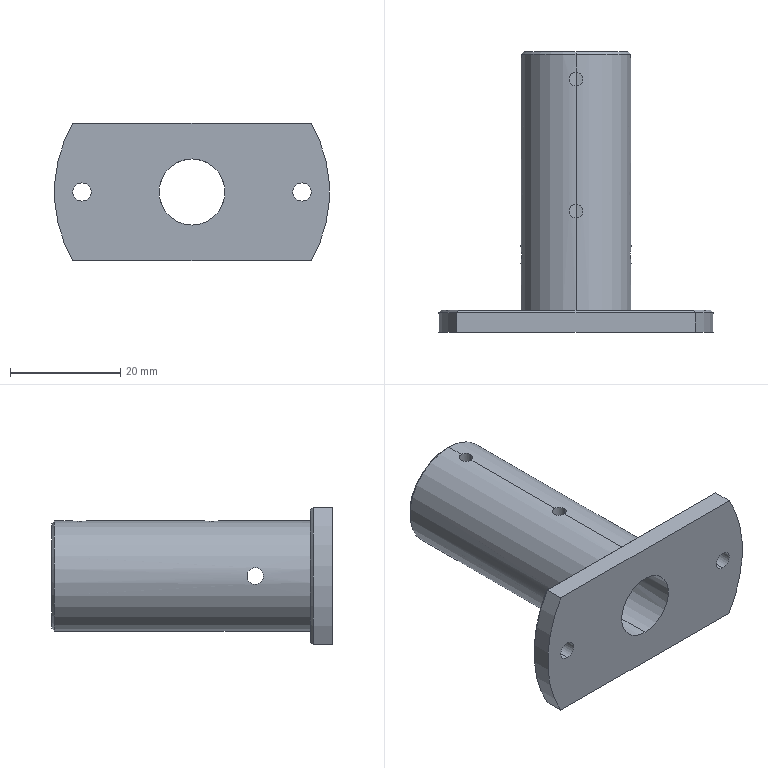Part | SolidWorks | features 3DProfileFeature 2, HoleWzd 2, ICE 2, Chamfer 1, Revolution 1 | 1 solid | 31 faces | box 50 x 51 x 25 mm | volume 13586 mm3 | cylinder 18 | plane 7 | cone 6 | commonest cylinder face diameters 2.5 x4 3 x4 3.3 x4 12 x2 20 x2 50 x2
STEP:
#1=CARTESIAN_POINT('',(-9.887,14.,1.5));
#2=VERTEX_POINT('',#1);
#3=CARTESIAN_POINT('',(-9.887,14.,-1.5));
#4=VERTEX_POINT('',#3);
#5=CARTESIAN_POINT('',(-9.887,14.,1.5));
#6=CARTESIAN_POINT('',(-9.887,13.804,1.5));
#7=CARTESIAN_POINT('',(-9.893,13.607,1.461));
#8=CARTESIAN_POINT('',(-9.914,13.245,1.311));
#9=CARTESIAN_POINT('',(-9.929,13.078,1.2));
#10=CARTESIAN_POINT('',(-9.951,12.871,0.9923));
#11=CARTESIAN_POINT('',(-9.958,12.808,0.9152));
#12=CARTESIAN_POINT('',(-9.972,12.699,0.7525));
#13=CARTESIAN_POINT('',(-9.978,12.653,0.6665));
#14=CARTESIAN_POINT('',(-9.994,12.539,0.394));
#15=CARTESIAN_POINT('',(-10.,12.5,0.1992));
#16=CARTESIAN_POINT('',(-10.,12.5,-0.09815));
#17=CARTESIAN_POINT('',(-9.999,12.51,-0.1957));
#18=CARTESIAN_POINT('',(-9.993,12.548,-0.3876));
#19=CARTESIAN_POINT('',(-9.989,12.577,-0.4831));
#20=CARTESIAN_POINT('',(-9.978,12.652,-0.6646));
#21=CARTESIAN_POINT('',(-9.972,12.698,-0.7507));
#22=CARTESIAN_POINT('',(-9.958,12.806,-0.9138));
#23=CARTESIAN_POINT('',(-9.951,12.87,-0.9909));
#24=CARTESIAN_POINT('',(-9.929,13.077,-1.198));
#25=CARTESIAN_POINT('',(-9.914,13.244,-1.31));
#26=CARTESIAN_POINT('',(-9.893,13.604,-1.46));
#27=CARTESIAN_POINT('',(-9.887,13.802,-1.5));
#28=CARTESIAN_POINT('',(-9.887,14.,-1.5));
#29=B_SPLINE_CURVE_WITH_KNOTS('',3,(#5,#6,#7,#8,#9,#10,#11,#12,#13,#14,#15,#16,#17,#18,#19,#20,#21,#22,#23,#24,#25,#26,#27,#28),.UNSPECIFIED.,.F.,.F.,(4,2,2,2,2,2,2,2,2,2,2,4),(0.004696,0.005283,0.00587,0.006164,0.006457,0.007044,0.007337,0.007631,0.007924,0.008218,0.008805,0.009391),.UNSPECIFIED.);
#30=EDGE_CURVE('',#2,#4,#29,.T.);
#31=ORIENTED_EDGE('',*,*,#30,.F.);
#32=CARTESIAN_POINT('',(-5.809,14.,1.5));
#33=VERTEX_POINT('',#32);
#34=CARTESIAN_POINT('',(-26.5,14.,1.5));
#35=DIRECTION('',(1.,0.,0.));
#36=VECTOR('',#35,1000.);
#37=LINE('',#34,#36);
#38=EDGE_CURVE('',#2,#33,#37,.T.);
#39=ORIENTED_EDGE('',*,*,#38,.T.);
#40=CARTESIAN_POINT('',(-5.809,14.,-1.5));
#41=VERTEX_POINT('',#40);
#42=CARTESIAN_POINT('',(-5.809,14.,-1.5));
#43=CARTESIAN_POINT('',(-5.809,13.9,-1.5));
#44=CARTESIAN_POINT('',(-5.812,13.803,-1.49));
#45=CARTESIAN_POINT('',(-5.822,13.61,-1.452));
#46=CARTESIAN_POINT('',(-5.829,13.515,-1.423));
#47=CARTESIAN_POINT('',(-5.847,13.333,-1.347));
#48=CARTESIAN_POINT('',(-5.857,13.247,-1.301));
#49=CARTESIAN_POINT('',(-5.881,13.085,-1.192));
#50=CARTESIAN_POINT('',(-5.893,13.008,-1.129));
#51=CARTESIAN_POINT('',(-5.93,12.801,-0.9226));
#52=CARTESIAN_POINT('',(-5.955,12.69,-0.7559));
#53=CARTESIAN_POINT('',(-5.99,12.54,-0.3951));
#54=CARTESIAN_POINT('',(-6.,12.5,-0.1972));
#55=CARTESIAN_POINT('',(-6.,12.5,0.09767));
#56=CARTESIAN_POINT('',(-5.998,12.51,0.1975));
#57=CARTESIAN_POINT('',(-5.988,12.548,0.3902));
#58=CARTESIAN_POINT('',(-5.981,12.577,0.4839));
#59=CARTESIAN_POINT('',(-5.955,12.69,0.7571));
#60=CARTESIAN_POINT('',(-5.93,12.801,0.922));
#61=CARTESIAN_POINT('',(-5.893,13.009,1.13));
#62=CARTESIAN_POINT('',(-5.881,13.084,1.192));
#63=CARTESIAN_POINT('',(-5.858,13.247,1.301));
#64=CARTESIAN_POINT('',(-5.847,13.335,1.348));
#65=CARTESIAN_POINT('',(-5.829,13.516,1.423));
#66=CARTESIAN_POINT('',(-5.822,13.609,1.452));
#67=CARTESIAN_POINT('',(-5.812,13.802,1.49));
#68=CARTESIAN_POINT('',(-5.809,13.902,1.5));
#69=CARTESIAN_POINT('',(-5.809,14.,1.5));
#70=B_SPLINE_CURVE_WITH_KNOTS('',3,(#42,#43,#44,#45,#46,#47,#48,#49,#50,#51,#52,#53,#54,#55,#56,#57,#58,#59,#60,#61,#62,#63,#64,#65,#66,#67,#68,#69),.UNSPECIFIED.,.F.,.F.,(4,2,2,2,2,2,2,2,2,2,2,2,2,4),(0.,0.0002943,0.0005885,0.0008828,0.001177,0.001766,0.002354,0.002648,0.002943,0.003531,0.003826,0.00412,0.004414,0.004708),.UNSPECIFIED.);
#71=EDGE_CURVE('',#41,#33,#70,.T.);
#72=ORIENTED_EDGE('',*,*,#71,.F.);
#73=CARTESIAN_POINT('',(-26.5,14.,-1.5));
#74=DIRECTION('',(1.,0.,0.));
#75=VECTOR('',#74,1000.);
#76=LINE('',#73,#75);
#77=EDGE_CURVE('',#4,#41,#76,.T.);
#78=ORIENTED_EDGE('',*,*,#77,.F.);
#79=EDGE_LOOP('',(#31,#39,#72,#78));
#80=FACE_OUTER_BOUND('',#79,.T.);
#81=CARTESIAN_POINT('',(-26.5,14.,0.));
#82=DIRECTION('',(1.,0.,0.));
#83=DIRECTION('',(0.,0.,-1.));
#84=AXIS2_PLACEMENT_3D('',#81,#82,#83);
#85=CYLINDRICAL_SURFACE('',#84,1.5);
#86=ADVANCED_FACE('',(#80),#85,.F.);
#87=CARTESIAN_POINT('',(5.809,14.,1.5));
#88=VERTEX_POINT('',#87);
#89=CARTESIAN_POINT('',(5.809,14.,-1.5));
#90=VERTEX_POINT('',#89);
#91=CARTESIAN_POINT('',(5.809,14.,1.5));
#92=CARTESIAN_POINT('',(5.809,13.804,1.5));
#93=CARTESIAN_POINT('',(5.82,13.606,1.46));
#94=CARTESIAN_POINT('',(5.847,13.335,1.348));
#95=CARTESIAN_POINT('',(5.858,13.247,1.301));
#96=CARTESIAN_POINT('',(5.881,13.084,1.192));
#97=CARTESIAN_POINT('',(5.893,13.009,1.13));
#98=CARTESIAN_POINT('',(5.918,12.871,0.9921));
#99=CARTESIAN_POINT('',(5.93,12.808,0.9153));
#100=CARTESIAN_POINT('',(5.953,12.699,0.7533));
#101=CARTESIAN_POINT('',(5.963,12.653,0.6673));
#102=CARTESIAN_POINT('',(5.99,12.539,0.3936));
#103=CARTESIAN_POINT('',(6.,12.5,0.1983));
#104=CARTESIAN_POINT('',(6.,12.5,-0.09848));
#105=CARTESIAN_POINT('',(5.998,12.51,-0.1961));
#106=CARTESIAN_POINT('',(5.988,12.548,-0.3888));
#107=CARTESIAN_POINT('',(5.981,12.577,-0.4845));
#108=CARTESIAN_POINT('',(5.955,12.69,-0.7559));
#109=CARTESIAN_POINT('',(5.93,12.801,-0.9224));
#110=CARTESIAN_POINT('',(5.881,13.076,-1.198));
#111=CARTESIAN_POINT('',(5.856,13.243,-1.31));
#112=CARTESIAN_POINT('',(5.829,13.514,-1.422));
#113=CARTESIAN_POINT('',(5.822,13.609,-1.452));
#114=CARTESIAN_POINT('',(5.812,13.802,-1.49));
#115=CARTESIAN_POINT('',(5.809,13.9,-1.5));
#116=CARTESIAN_POINT('',(5.809,14.,-1.5));
#117=B_SPLINE_CURVE_WITH_KNOTS('',3,(#91,#92,#93,#94,#95,#96,#97,#98,#99,#100,#101,#102,#103,#104,#105,#106,#107,#108,#109,#110,#111,#112,#113,#114,#115,#116),.UNSPECIFIED.,.F.,.F.,(4,2,2,2,2,2,2,2,2,2,2,2,4),(0.004708,0.005297,0.005591,0.005885,0.006179,0.006474,0.007062,0.007356,0.00765,0.008239,0.008827,0.009121,0.009415),.UNSPECIFIED.);
#118=EDGE_CURVE('',#88,#90,#117,.T.);
#119=ORIENTED_EDGE('',*,*,#118,.F.);
#120=CARTESIAN_POINT('',(9.887,14.,1.5));
#121=VERTEX_POINT('',#120);
#122=CARTESIAN_POINT('',(-26.5,14.,1.5));
#123=DIRECTION('',(1.,0.,0.));
#124=VECTOR('',#123,1000.);
#125=LINE('',#122,#124);
#126=EDGE_CURVE('',#88,#121,#125,.T.);
#127=ORIENTED_EDGE('',*,*,#126,.T.);
#128=CARTESIAN_POINT('',(9.887,14.,-1.5));
#129=VERTEX_POINT('',#128);
#130=CARTESIAN_POINT('',(9.887,14.,-1.5));
#131=CARTESIAN_POINT('',(9.887,13.901,-1.5));
#132=CARTESIAN_POINT('',(9.888,13.803,-1.49));
#133=CARTESIAN_POINT('',(9.894,13.611,-1.452));
#134=CARTESIAN_POINT('',(9.898,13.516,-1.423));
#135=CARTESIAN_POINT('',(9.909,13.334,-1.348));
#136=CARTESIAN_POINT('',(9.915,13.248,-1.302));
#137=CARTESIAN_POINT('',(9.929,13.085,-1.193));
#138=CARTESIAN_POINT('',(9.936,13.008,-1.13));
#139=CARTESIAN_POINT('',(9.958,12.801,-0.9222));
#140=CARTESIAN_POINT('',(9.973,12.689,-0.7551));
#141=CARTESIAN_POINT('',(9.994,12.54,-0.3942));
#142=CARTESIAN_POINT('',(10.,12.5,-0.1965));
#143=CARTESIAN_POINT('',(10.,12.5,0.09743));
#144=CARTESIAN_POINT('',(9.999,12.51,0.197));
#145=CARTESIAN_POINT('',(9.993,12.548,0.3895));
#146=CARTESIAN_POINT('',(9.989,12.577,0.4831));
#147=CARTESIAN_POINT('',(9.973,12.689,0.7557));
#148=CARTESIAN_POINT('',(9.959,12.8,0.9208));
#149=CARTESIAN_POINT('',(9.936,13.009,1.131));
#150=CARTESIAN_POINT('',(9.929,13.085,1.192));
#151=CARTESIAN_POINT('',(9.915,13.247,1.301));
#152=CARTESIAN_POINT('',(9.909,13.335,1.348));
#153=CARTESIAN_POINT('',(9.898,13.516,1.423));
#154=CARTESIAN_POINT('',(9.894,13.61,1.452));
#155=CARTESIAN_POINT('',(9.888,13.803,1.49));
#156=CARTESIAN_POINT('',(9.887,13.902,1.5));
#157=CARTESIAN_POINT('',(9.887,14.,1.5));
#158=B_SPLINE_CURVE_WITH_KNOTS('',3,(#130,#131,#132,#133,#134,#135,#136,#137,#138,#139,#140,#141,#142,#143,#144,#145,#146,#147,#148,#149,#150,#151,#152,#153,#154,#155,#156,#157),.UNSPECIFIED.,.F.,.F.,(4,2,2,2,2,2,2,2,2,2,2,2,2,4),(0.,0.0002935,0.000587,0.0008806,0.001174,0.001761,0.002348,0.002642,0.002935,0.003522,0.003816,0.004109,0.004403,0.004696),.UNSPECIFIED.);
#159=EDGE_CURVE('',#129,#121,#158,.T.);
#160=ORIENTED_EDGE('',*,*,#159,.F.);
#161=CARTESIAN_POINT('',(-26.5,14.,-1.5));
#162=DIRECTION('',(1.,0.,0.));
#163=VECTOR('',#162,1000.);
#164=LINE('',#161,#163);
#165=EDGE_CURVE('',#90,#129,#164,.T.);
#166=ORIENTED_EDGE('',*,*,#165,.F.);
#167=EDGE_LOOP('',(#119,#127,#160,#166));
#168=FACE_OUTER_BOUND('',#167,.T.);
#169=CARTESIAN_POINT('',(-26.5,14.,0.));
#170=DIRECTION('',(1.,0.,0.));
#171=DIRECTION('',(0.,0.,-1.));
#172=AXIS2_PLACEMENT_3D('',#169,#170,#171);
#173=CYLINDRICAL_SURFACE('',#172,1.5);
#174=ADVANCED_FACE('',(#168),#173,.F.);
#175=CARTESIAN_POINT('',(-20.,4.,1.65));
#176=VERTEX_POINT('',#175);
#177=CARTESIAN_POINT('',(-20.,4.,-1.65));
#178=VERTEX_POINT('',#177);
#179=CARTESIAN_POINT('',(-20.,4.,0.));
#180=DIRECTION('',(0.,-1.,0.));
#181=DIRECTION('',(0.,0.,-1.));
#182=AXIS2_PLACEMENT_3D('',#179,#180,#181);
#183=CIRCLE('',#182,1.65);
#184=EDGE_CURVE('',#176,#178,#183,.T.);
#185=ORIENTED_EDGE('',*,*,#184,.F.);
#186=CARTESIAN_POINT('',(-20.,0.,1.65));
#187=VERTEX_POINT('',#186);
#188=CARTESIAN_POINT('',(-20.,0.,1.65));
#189=DIRECTION('',(0.,-1.,0.));
#190=VECTOR('',#189,1000.);
#191=LINE('',#188,#190);
#192=EDGE_CURVE('',#176,#187,#191,.T.);
#193=ORIENTED_EDGE('',*,*,#192,.T.);
#194=CARTESIAN_POINT('',(-20.,0.,-1.65));
#195=VERTEX_POINT('',#194);
#196=CARTESIAN_POINT('',(-20.,0.,0.));
#197=DIRECTION('',(0.,-1.,0.));
#198=DIRECTION('',(0.,0.,-1.));
#199=AXIS2_PLACEMENT_3D('',#196,#197,#198);
#200=CIRCLE('',#199,1.65);
#201=EDGE_CURVE('',#187,#195,#200,.T.);
#202=ORIENTED_EDGE('',*,*,#201,.T.);
#203=CARTESIAN_POINT('',(-20.,0.,-1.65));
#204=DIRECTION('',(0.,-1.,0.));
#205=VECTOR('',#204,1000.);
#206=LINE('',#203,#205);
#207=EDGE_CURVE('',#178,#195,#206,.T.);
#208=ORIENTED_EDGE('',*,*,#207,.F.);
#209=EDGE_LOOP('',(#185,#193,#202,#208));
#210=FACE_OUTER_BOUND('',#209,.T.);
#211=CARTESIAN_POINT('',(-20.,0.,0.));
#212=DIRECTION('',(0.,-1.,0.));
#213=DIRECTION('',(0.,0.,-1.));
#214=AXIS2_PLACEMENT_3D('',#211,#212,#213);
#215=CYLINDRICAL_SURFACE('',#214,1.65);
#216=ADVANCED_FACE('',(#210),#215,.F.);
#217=CARTESIAN_POINT('',(20.,4.,1.65));
#218=VERTEX_POINT('',#217);
#219=CARTESIAN_POINT('',(20.,4.,-1.65));
#220=VERTEX_POINT('',#219);
#221=CARTESIAN_POINT('',(20.,4.,0.));
#222=DIRECTION('',(0.,-1.,0.));
#223=DIRECTION('',(0.,0.,-1.));
#224=AXIS2_PLACEMENT_3D('',#221,#222,#223);
#225=CIRCLE('',#224,1.65);
#226=EDGE_CURVE('',#218,#220,#225,.T.);
#227=ORIENTED_EDGE('',*,*,#226,.F.);
#228=CARTESIAN_POINT('',(20.,0.,1.65));
#229=VERTEX_POINT('',#228);
#230=CARTESIAN_POINT('',(20.,0.,1.65));
#231=DIRECTION('',(0.,-1.,0.));
#232=VECTOR('',#231,1000.);
#233=LINE('',#230,#232);
#234=EDGE_CURVE('',#218,#229,#233,.T.);
#235=ORIENTED_EDGE('',*,*,#234,.T.);
#236=CARTESIAN_POINT('',(20.,0.,-1.65));
#237=VERTEX_POINT('',#236);
#238=CARTESIAN_POINT('',(20.,0.,0.));
#239=DIRECTION('',(0.,-1.,0.));
#240=DIRECTION('',(0.,0.,-1.));
#241=AXIS2_PLACEMENT_3D('',#238,#239,#240);
#242=CIRCLE('',#241,1.65);
#243=EDGE_CURVE('',#229,#237,#242,.T.);
#244=ORIENTED_EDGE('',*,*,#243,.T.);
#245=CARTESIAN_POINT('',(20.,0.,-1.65));
#246=DIRECTION('',(0.,-1.,0.));
#247=VECTOR('',#246,1000.);
#248=LINE('',#245,#247);
#249=EDGE_CURVE('',#220,#237,#248,.T.);
#250=ORIENTED_EDGE('',*,*,#249,.F.);
#251=EDGE_LOOP('',(#227,#235,#244,#250));
#252=FACE_OUTER_BOUND('',#251,.T.);
#253=CARTESIAN_POINT('',(20.,0.,0.));
#254=DIRECTION('',(0.,-1.,0.));
#255=DIRECTION('',(0.,0.,-1.));
#256=AXIS2_PLACEMENT_3D('',#253,#254,#255);
#257=CYLINDRICAL_SURFACE('',#256,1.65);
#258=ADVANCED_FACE('',(#252),#257,.F.);
#259=CARTESIAN_POINT('',(-1.25,22.,5.868));
#260=VERTEX_POINT('',#259);
#261=CARTESIAN_POINT('',(0.,20.75,6.));
#262=VERTEX_POINT('',#261);
#263=CARTESIAN_POINT('',(-1.25,22.,5.868));
#264=CARTESIAN_POINT('',(-1.25,21.835,5.868));
#265=CARTESIAN_POINT('',(-1.217,21.672,5.876));
#266=CARTESIAN_POINT('',(-1.092,21.37,5.9));
#267=CARTESIAN_POINT('',(-0.999,21.231,5.917));
#268=CARTESIAN_POINT('',(-0.7695,21.002,5.952));
#269=CARTESIAN_POINT('',(-0.6305,20.908,5.969));
#270=CARTESIAN_POINT('',(-0.3299,20.783,5.993));
#271=CARTESIAN_POINT('',(-0.1656,20.75,6.));
#272=CARTESIAN_POINT('',(0.,20.75,6.));
#273=B_SPLINE_CURVE_WITH_KNOTS('',3,(#263,#264,#265,#266,#267,#268,#269,#270,#271,#272),.UNSPECIFIED.,.F.,.F.,(4,2,2,2,4),(0.005878,0.006368,0.006857,0.007347,0.007837),.UNSPECIFIED.);
#274=EDGE_CURVE('',#260,#262,#273,.T.);
#275=ORIENTED_EDGE('',*,*,#274,.F.);
#276=CARTESIAN_POINT('',(-1.25,22.,9.922));
#277=VERTEX_POINT('',#276);
#278=CARTESIAN_POINT('',(-1.25,22.,10.));
#279=DIRECTION('',(0.,0.,1.));
#280=VECTOR('',#279,1000.);
#281=LINE('',#278,#280);
#282=EDGE_CURVE('',#260,#277,#281,.T.);
#283=ORIENTED_EDGE('',*,*,#282,.T.);
#284=CARTESIAN_POINT('',(0.,20.75,10.));
#285=VERTEX_POINT('',#284);
#286=CARTESIAN_POINT('',(0.,20.75,10.));
#287=CARTESIAN_POINT('',(-0.1654,20.75,10.));
#288=CARTESIAN_POINT('',(-0.3277,20.783,9.996));
#289=CARTESIAN_POINT('',(-0.6304,20.908,9.981));
#290=CARTESIAN_POINT('',(-0.769,21.001,9.971));
#291=CARTESIAN_POINT('',(-0.9994,21.232,9.951));
#292=CARTESIAN_POINT('',(-1.093,21.371,9.94));
#293=CARTESIAN_POINT('',(-1.217,21.672,9.926));
#294=CARTESIAN_POINT('',(-1.25,21.837,9.922));
#295=CARTESIAN_POINT('',(-1.25,22.,9.922));
#296=B_SPLINE_CURVE_WITH_KNOTS('',3,(#286,#287,#288,#289,#290,#291,#292,#293,#294,#295),.UNSPECIFIED.,.F.,.F.,(4,2,2,2,4),(0.,0.0004891,0.0009782,0.001467,0.001956),.UNSPECIFIED.);
#297=EDGE_CURVE('',#285,#277,#296,.T.);
#298=ORIENTED_EDGE('',*,*,#297,.F.);
#299=CARTESIAN_POINT('',(1.25,22.,9.922));
#300=VERTEX_POINT('',#299);
#301=CARTESIAN_POINT('',(1.25,22.,9.922));
#302=CARTESIAN_POINT('',(1.25,21.835,9.922));
#303=CARTESIAN_POINT('',(1.217,21.673,9.926));
#304=CARTESIAN_POINT('',(1.092,21.37,9.94));
#305=CARTESIAN_POINT('',(0.9993,21.232,9.951));
#306=CARTESIAN_POINT('',(0.7691,21.001,9.971));
#307=CARTESIAN_POINT('',(0.6299,20.908,9.981));
#308=CARTESIAN_POINT('',(0.3294,20.783,9.996));
#309=CARTESIAN_POINT('',(0.1652,20.75,10.));
#310=CARTESIAN_POINT('',(0.,20.75,10.));
#311=B_SPLINE_CURVE_WITH_KNOTS('',3,(#301,#302,#303,#304,#305,#306,#307,#308,#309,#310),.UNSPECIFIED.,.F.,.F.,(4,2,2,2,4),(0.005868,0.006357,0.006846,0.007334,0.007823),.UNSPECIFIED.);
#312=EDGE_CURVE('',#300,#285,#311,.T.);
#313=ORIENTED_EDGE('',*,*,#312,.F.);
#314=CARTESIAN_POINT('',(1.25,22.,5.868));
#315=VERTEX_POINT('',#314);
#316=CARTESIAN_POINT('',(1.25,22.,10.));
#317=DIRECTION('',(0.,0.,1.));
#318=VECTOR('',#317,1000.);
#319=LINE('',#316,#318);
#320=EDGE_CURVE('',#315,#300,#319,.T.);
#321=ORIENTED_EDGE('',*,*,#320,.F.);
#322=CARTESIAN_POINT('',(0.,20.75,6.));
#323=CARTESIAN_POINT('',(0.1657,20.75,6.));
#324=CARTESIAN_POINT('',(0.3283,20.783,5.993));
#325=CARTESIAN_POINT('',(0.6309,20.909,5.969));
#326=CARTESIAN_POINT('',(0.7693,21.001,5.952));
#327=CARTESIAN_POINT('',(0.9992,21.232,5.917));
#328=CARTESIAN_POINT('',(1.092,21.371,5.9));
#329=CARTESIAN_POINT('',(1.217,21.672,5.876));
#330=CARTESIAN_POINT('',(1.25,21.836,5.868));
#331=CARTESIAN_POINT('',(1.25,22.,5.868));
#332=B_SPLINE_CURVE_WITH_KNOTS('',3,(#322,#323,#324,#325,#326,#327,#328,#329,#330,#331),.UNSPECIFIED.,.F.,.F.,(4,2,2,2,4),(0.,0.00049,0.00098,0.00147,0.00196),.UNSPECIFIED.);
#333=EDGE_CURVE('',#262,#315,#332,.T.);
#334=ORIENTED_EDGE('',*,*,#333,.F.);
#335=EDGE_LOOP('',(#275,#283,#298,#313,#321,#334));
#336=FACE_OUTER_BOUND('',#335,.T.);
#337=CARTESIAN_POINT('',(0.,22.,10.));
#338=DIRECTION('',(0.,0.,1.));
#339=DIRECTION('',(1.,0.,0.));
#340=AXIS2_PLACEMENT_3D('',#337,#338,#339);
#341=CYLINDRICAL_SURFACE('',#340,1.25);
#342=ADVANCED_FACE('',(#336),#341,.F.);
#343=CARTESIAN_POINT('',(-1.25,46.,5.868));
#344=VERTEX_POINT('',#343);
#345=CARTESIAN_POINT('',(0.,44.75,6.));
#346=VERTEX_POINT('',#345);
#347=CARTESIAN_POINT('',(-1.25,46.,5.868));
#348=CARTESIAN_POINT('',(-1.25,45.835,5.868));
#349=CARTESIAN_POINT('',(-1.217,45.672,5.876));
#350=CARTESIAN_POINT('',(-1.092,45.37,5.9));
#351=CARTESIAN_POINT('',(-0.999,45.231,5.917));
#352=CARTESIAN_POINT('',(-0.7695,45.002,5.952));
#353=CARTESIAN_POINT('',(-0.6305,44.908,5.969));
#354=CARTESIAN_POINT('',(-0.3299,44.783,5.993));
#355=CARTESIAN_POINT('',(-0.1656,44.75,6.));
#356=CARTESIAN_POINT('',(0.,44.75,6.));
#357=B_SPLINE_CURVE_WITH_KNOTS('',3,(#347,#348,#349,#350,#351,#352,#353,#354,#355,#356),.UNSPECIFIED.,.F.,.F.,(4,2,2,2,4),(0.005878,0.006368,0.006857,0.007347,0.007837),.UNSPECIFIED.);
#358=EDGE_CURVE('',#344,#346,#357,.T.);
#359=ORIENTED_EDGE('',*,*,#358,.F.);
#360=CARTESIAN_POINT('',(-1.25,46.,9.922));
#361=VERTEX_POINT('',#360);
#362=CARTESIAN_POINT('',(-1.25,46.,10.));
#363=DIRECTION('',(0.,0.,1.));
#364=VECTOR('',#363,1000.);
#365=LINE('',#362,#364);
#366=EDGE_CURVE('',#344,#361,#365,.T.);
#367=ORIENTED_EDGE('',*,*,#366,.T.);
#368=CARTESIAN_POINT('',(0.,44.75,10.));
#369=VERTEX_POINT('',#368);
#370=CARTESIAN_POINT('',(0.,44.75,10.));
#371=CARTESIAN_POINT('',(-0.1654,44.75,10.));
#372=CARTESIAN_POINT('',(-0.3277,44.783,9.996));
#373=CARTESIAN_POINT('',(-0.6304,44.908,9.981));
#374=CARTESIAN_POINT('',(-0.769,45.001,9.971));
#375=CARTESIAN_POINT('',(-0.9994,45.232,9.951));
#376=CARTESIAN_POINT('',(-1.093,45.371,9.94));
#377=CARTESIAN_POINT('',(-1.217,45.672,9.926));
#378=CARTESIAN_POINT('',(-1.25,45.837,9.922));
#379=CARTESIAN_POINT('',(-1.25,46.,9.922));
#380=B_SPLINE_CURVE_WITH_KNOTS('',3,(#370,#371,#372,#373,#374,#375,#376,#377,#378,#379),.UNSPECIFIED.,.F.,.F.,(4,2,2,2,4),(0.,0.0004891,0.0009782,0.001467,0.001956),.UNSPECIFIED.);
#381=EDGE_CURVE('',#369,#361,#380,.T.);
#382=ORIENTED_EDGE('',*,*,#381,.F.);
#383=CARTESIAN_POINT('',(1.25,46.,9.922));
#384=VERTEX_POINT('',#383);
#385=CARTESIAN_POINT('',(1.25,46.,9.922));
#386=CARTESIAN_POINT('',(1.25,45.835,9.922));
#387=CARTESIAN_POINT('',(1.217,45.673,9.926));
#388=CARTESIAN_POINT('',(1.092,45.37,9.94));
#389=CARTESIAN_POINT('',(0.9993,45.232,9.951));
#390=CARTESIAN_POINT('',(0.7691,45.001,9.971));
#391=CARTESIAN_POINT('',(0.6299,44.908,9.981));
#392=CARTESIAN_POINT('',(0.3294,44.783,9.996));
#393=CARTESIAN_POINT('',(0.1652,44.75,10.));
#394=CARTESIAN_POINT('',(0.,44.75,10.));
#395=B_SPLINE_CURVE_WITH_KNOTS('',3,(#385,#386,#387,#388,#389,#390,#391,#392,#393,#394),.UNSPECIFIED.,.F.,.F.,(4,2,2,2,4),(0.005868,0.006357,0.006846,0.007334,0.007823),.UNSPECIFIED.);
#396=EDGE_CURVE('',#384,#369,#395,.T.);
#397=ORIENTED_EDGE('',*,*,#396,.F.);
#398=CARTESIAN_POINT('',(1.25,46.,5.868));
#399=VERTEX_POINT('',#398);
#400=CARTESIAN_POINT('',(1.25,46.,10.));
#401=DIRECTION('',(0.,0.,1.));
#402=VECTOR('',#401,1000.);
#403=LINE('',#400,#402);
#404=EDGE_CURVE('',#399,#384,#403,.T.);
#405=ORIENTED_EDGE('',*,*,#404,.F.);
#406=CARTESIAN_POINT('',(0.,44.75,6.));
#407=CARTESIAN_POINT('',(0.1657,44.75,6.));
#408=CARTESIAN_POINT('',(0.3283,44.783,5.993));
#409=CARTESIAN_POINT('',(0.6309,44.909,5.969));
#410=CARTESIAN_POINT('',(0.7693,45.001,5.952));
#411=CARTESIAN_POINT('',(0.9992,45.232,5.917));
#412=CARTESIAN_POINT('',(1.092,45.371,5.9));
#413=CARTESIAN_POINT('',(1.217,45.672,5.876));
#414=CARTESIAN_POINT('',(1.25,45.836,5.868));
#415=CARTESIAN_POINT('',(1.25,46.,5.868));
#416=B_SPLINE_CURVE_WITH_KNOTS('',3,(#406,#407,#408,#409,#410,#411,#412,#413,#414,#415),.UNSPECIFIED.,.F.,.F.,(4,2,2,2,4),(0.,0.00049,0.00098,0.00147,0.00196),.UNSPECIFIED.);
#417=EDGE_CURVE('',#346,#399,#416,.T.);
#418=ORIENTED_EDGE('',*,*,#417,.F.);
#419=EDGE_LOOP('',(#359,#367,#382,#397,#405,#418));
#420=FACE_OUTER_BOUND('',#419,.T.);
#421=CARTESIAN_POINT('',(0.,46.,10.));
#422=DIRECTION('',(0.,0.,1.));
#423=DIRECTION('',(1.,0.,0.));
#424=AXIS2_PLACEMENT_3D('',#421,#422,#423);
#425=CYLINDRICAL_SURFACE('',#424,1.25);
#426=ADVANCED_FACE('',(#420),#425,.F.);
#427=CARTESIAN_POINT('',(0.,51.,9.5));
#428=VERTEX_POINT('',#427);
#429=CARTESIAN_POINT('',(0.,51.,-9.5));
#430=VERTEX_POINT('',#429);
#431=CARTESIAN_POINT('',(0.,51.,0.));
#432=DIRECTION('',(0.,1.,0.));
#433=DIRECTION('',(0.,0.,-1.));
#434=AXIS2_PLACEMENT_3D('',#431,#432,#433);
#435=CIRCLE('',#434,9.5);
#436=EDGE_CURVE('',#428,#430,#435,.T.);
#437=ORIENTED_EDGE('',*,*,#436,.F.);
#438=CARTESIAN_POINT('',(0.,50.5,10.));
#439=VERTEX_POINT('',#438);
#440=CARTESIAN_POINT('',(0.,51.,9.5));
#441=DIRECTION('',(0.,-0.7071,0.7071));
#442=VECTOR('',#441,1000.);
#443=LINE('',#440,#442);
#444=EDGE_CURVE('',#428,#439,#443,.T.);
#445=ORIENTED_EDGE('',*,*,#444,.T.);
#446=CARTESIAN_POINT('',(0.,50.5,-10.));
#447=VERTEX_POINT('',#446);
#448=CARTESIAN_POINT('',(0.,50.5,0.));
#449=DIRECTION('',(0.,-1.,0.));
#450=DIRECTION('',(0.,0.,-1.));
#451=AXIS2_PLACEMENT_3D('',#448,#449,#450);
#452=CIRCLE('',#451,10.);
#453=EDGE_CURVE('',#447,#439,#452,.T.);
#454=ORIENTED_EDGE('',*,*,#453,.F.);
#455=CARTESIAN_POINT('',(0.,51.,-9.5));
#456=DIRECTION('',(0.,-0.7071,-0.7071));
#457=VECTOR('',#456,1000.);
#458=LINE('',#455,#457);
#459=EDGE_CURVE('',#430,#447,#458,.T.);
#460=ORIENTED_EDGE('',*,*,#459,.F.);
#461=EDGE_LOOP('',(#437,#445,#454,#460));
#462=FACE_OUTER_BOUND('',#461,.T.);
#463=CARTESIAN_POINT('',(0.,51.,0.));
#464=DIRECTION('',(0.,-1.,0.));
#465=DIRECTION('',(0.,0.,-1.));
#466=AXIS2_PLACEMENT_3D('',#463,#464,#465);
#467=CONICAL_SURFACE('',#466,9.5,0.7854);
#468=ADVANCED_FACE('',(#462),#467,.T.);
#469=CARTESIAN_POINT('',(0.,50.5,-6.));
#470=VERTEX_POINT('',#469);
#471=CARTESIAN_POINT('',(0.,50.5,6.));
#472=VERTEX_POINT('',#471);
#473=CARTESIAN_POINT('',(0.,50.5,0.));
#474=DIRECTION('',(0.,1.,0.));
#475=DIRECTION('',(0.,0.,-1.));
#476=AXIS2_PLACEMENT_3D('',#473,#474,#475);
#477=CIRCLE('',#476,6.);
#478=EDGE_CURVE('',#470,#472,#477,.T.);
#479=ORIENTED_EDGE('',*,*,#478,.F.);
#480=CARTESIAN_POINT('',(0.,51.,-6.5));
#481=VERTEX_POINT('',#480);
#482=CARTESIAN_POINT('',(0.,50.5,-6.));
#483=DIRECTION('',(0.,0.7071,-0.7071));
#484=VECTOR('',#483,1000.);
#485=LINE('',#482,#484);
#486=EDGE_CURVE('',#470,#481,#485,.T.);
#487=ORIENTED_EDGE('',*,*,#486,.T.);
#488=CARTESIAN_POINT('',(0.,51.,6.5));
#489=VERTEX_POINT('',#488);
#490=CARTESIAN_POINT('',(0.,51.,0.));
#491=DIRECTION('',(0.,-1.,0.));
#492=DIRECTION('',(0.,0.,-1.));
#493=AXIS2_PLACEMENT_3D('',#490,#491,#492);
#494=CIRCLE('',#493,6.5);
#495=EDGE_CURVE('',#489,#481,#494,.T.);
#496=ORIENTED_EDGE('',*,*,#495,.F.);
#497=CARTESIAN_POINT('',(0.,50.5,6.));
#498=DIRECTION('',(0.,0.7071,0.7071));
#499=VECTOR('',#498,1000.);
#500=LINE('',#497,#499);
#501=EDGE_CURVE('',#472,#489,#500,.T.);
#502=ORIENTED_EDGE('',*,*,#501,.F.);
#503=EDGE_LOOP('',(#479,#487,#496,#502));
#504=FACE_OUTER_BOUND('',#503,.T.);
#505=CARTESIAN_POINT('',(0.,50.5,0.));
#506=DIRECTION('',(0.,1.,0.));
#507=DIRECTION('',(0.,0.,1.));
#508=AXIS2_PLACEMENT_3D('',#505,#506,#507);
#509=CONICAL_SURFACE('',#508,6.,0.7854);
#510=ADVANCED_FACE('',(#504),#509,.F.);
#511=ORIENTED_EDGE('',*,*,#71,.T.);
#512=CARTESIAN_POINT('',(-5.809,14.,1.5));
#513=CARTESIAN_POINT('',(-5.809,14.196,1.5));
#514=CARTESIAN_POINT('',(-5.82,14.394,1.46));
#515=CARTESIAN_POINT('',(-5.847,14.665,1.348));
#516=CARTESIAN_POINT('',(-5.858,14.753,1.301));
#517=CARTESIAN_POINT('',(-5.881,14.916,1.192));
#518=CARTESIAN_POINT('',(-5.893,14.991,1.13));
#519=CARTESIAN_POINT('',(-5.918,15.129,0.9921));
#520=CARTESIAN_POINT('',(-5.93,15.192,0.9153));
#521=CARTESIAN_POINT('',(-5.953,15.301,0.7533));
#522=CARTESIAN_POINT('',(-5.963,15.347,0.6673));
#523=CARTESIAN_POINT('',(-5.99,15.461,0.3936));
#524=CARTESIAN_POINT('',(-6.,15.5,0.1983));
#525=CARTESIAN_POINT('',(-6.,15.5,-0.09848));
#526=CARTESIAN_POINT('',(-5.998,15.49,-0.1961));
#527=CARTESIAN_POINT('',(-5.988,15.452,-0.3888));
#528=CARTESIAN_POINT('',(-5.981,15.423,-0.4845));
#529=CARTESIAN_POINT('',(-5.955,15.31,-0.7559));
#530=CARTESIAN_POINT('',(-5.93,15.199,-0.9224));
#531=CARTESIAN_POINT('',(-5.881,14.924,-1.198));
#532=CARTESIAN_POINT('',(-5.856,14.757,-1.31));
#533=CARTESIAN_POINT('',(-5.829,14.486,-1.422));
#534=CARTESIAN_POINT('',(-5.822,14.391,-1.452));
#535=CARTESIAN_POINT('',(-5.812,14.198,-1.49));
#536=CARTESIAN_POINT('',(-5.809,14.1,-1.5));
#537=CARTESIAN_POINT('',(-5.809,14.,-1.5));
#538=B_SPLINE_CURVE_WITH_KNOTS('',3,(#512,#513,#514,#515,#516,#517,#518,#519,#520,#521,#522,#523,#524,#525,#526,#527,#528,#529,#530,#531,#532,#533,#534,#535,#536,#537),.UNSPECIFIED.,.F.,.F.,(4,2,2,2,2,2,2,2,2,2,2,2,4),(0.004708,0.005297,0.005591,0.005885,0.006179,0.006474,0.007062,0.007356,0.00765,0.008239,0.008827,0.009121,0.009415),.UNSPECIFIED.);
#539=EDGE_CURVE('',#33,#41,#538,.T.);
#540=ORIENTED_EDGE('',*,*,#539,.T.);
#541=EDGE_LOOP('',(#511,#540));
#542=FACE_BOUND('',#541,.T.);
#543=CARTESIAN_POINT('',(0.,0.,-6.));
#544=VERTEX_POINT('',#543);
#545=CARTESIAN_POINT('',(0.,0.,6.));
#546=VERTEX_POINT('',#545);
#547=CARTESIAN_POINT('',(0.,0.,0.));
#548=DIRECTION('',(0.,1.,0.));
#549=DIRECTION('',(0.,0.,1.));
#550=AXIS2_PLACEMENT_3D('',#547,#548,#549);
#551=CIRCLE('',#550,6.);
#552=EDGE_CURVE('',#544,#546,#551,.T.);
#553=ORIENTED_EDGE('',*,*,#552,.F.);
#554=CARTESIAN_POINT('',(0.,57.583,-6.));
#555=DIRECTION('',(0.,1.,0.));
#556=VECTOR('',#555,1000.);
#557=LINE('',#554,#556);
#558=EDGE_CURVE('',#544,#470,#557,.T.);
#559=ORIENTED_EDGE('',*,*,#558,.T.);
#560=ORIENTED_EDGE('',*,*,#478,.T.);
#561=CARTESIAN_POINT('',(0.,47.25,6.));
#562=VERTEX_POINT('',#561);
#563=CARTESIAN_POINT('',(0.,57.583,6.));
#564=DIRECTION('',(0.,1.,0.));
#565=VECTOR('',#564,1000.);
#566=LINE('',#563,#565);
#567=EDGE_CURVE('',#562,#472,#566,.T.);
#568=ORIENTED_EDGE('',*,*,#567,.F.);
#569=CARTESIAN_POINT('',(0.,47.25,6.));
#570=CARTESIAN_POINT('',(-0.1634,47.25,6.));
#571=CARTESIAN_POINT('',(-0.3284,47.217,5.993));
#572=CARTESIAN_POINT('',(-0.6294,47.092,5.969));
#573=CARTESIAN_POINT('',(-0.7683,46.999,5.952));
#574=CARTESIAN_POINT('',(-0.9989,46.769,5.917));
#575=CARTESIAN_POINT('',(-1.091,46.631,5.9));
#576=CARTESIAN_POINT('',(-1.217,46.328,5.876));
#577=CARTESIAN_POINT('',(-1.25,46.165,5.868));
#578=CARTESIAN_POINT('',(-1.25,46.,5.868));
#579=B_SPLINE_CURVE_WITH_KNOTS('',3,(#569,#570,#571,#572,#573,#574,#575,#576,#577,#578),.UNSPECIFIED.,.F.,.F.,(4,2,2,2,4),(0.003919,0.004409,0.004899,0.005388,0.005878),.UNSPECIFIED.);
#580=EDGE_CURVE('',#562,#344,#579,.T.);
#581=ORIENTED_EDGE('',*,*,#580,.T.);
#582=ORIENTED_EDGE('',*,*,#358,.T.);
#583=CARTESIAN_POINT('',(0.,23.25,6.));
#584=VERTEX_POINT('',#583);
#585=CARTESIAN_POINT('',(0.,57.583,6.));
#586=DIRECTION('',(0.,1.,0.));
#587=VECTOR('',#586,1000.);
#588=LINE('',#585,#587);
#589=EDGE_CURVE('',#584,#346,#588,.T.);
#590=ORIENTED_EDGE('',*,*,#589,.F.);
#591=CARTESIAN_POINT('',(0.,23.25,6.));
#592=CARTESIAN_POINT('',(-0.1634,23.25,6.));
#593=CARTESIAN_POINT('',(-0.3284,23.217,5.993));
#594=CARTESIAN_POINT('',(-0.6294,23.092,5.969));
#595=CARTESIAN_POINT('',(-0.7683,22.999,5.952));
#596=CARTESIAN_POINT('',(-0.9989,22.769,5.917));
#597=CARTESIAN_POINT('',(-1.091,22.631,5.9));
#598=CARTESIAN_POINT('',(-1.217,22.328,5.876));
#599=CARTESIAN_POINT('',(-1.25,22.165,5.868));
#600=CARTESIAN_POINT('',(-1.25,22.,5.868));
#601=B_SPLINE_CURVE_WITH_KNOTS('',3,(#591,#592,#593,#594,#595,#596,#597,#598,#599,#600),.UNSPECIFIED.,.F.,.F.,(4,2,2,2,4),(0.003919,0.004409,0.004899,0.005388,0.005878),.UNSPECIFIED.);
#602=EDGE_CURVE('',#584,#260,#601,.T.);
#603=ORIENTED_EDGE('',*,*,#602,.T.);
#604=ORIENTED_EDGE('',*,*,#274,.T.);
#605=CARTESIAN_POINT('',(0.,57.583,6.));
#606=DIRECTION('',(0.,1.,0.));
#607=VECTOR('',#606,1000.);
#608=LINE('',#605,#607);
#609=EDGE_CURVE('',#546,#262,#608,.T.);
#610=ORIENTED_EDGE('',*,*,#609,.F.);
#611=EDGE_LOOP('',(#553,#559,#560,#568,#581,#582,#590,#603,#604,#610));
#612=FACE_OUTER_BOUND('',#611,.T.);
#613=CARTESIAN_POINT('',(0.,57.583,0.));
#614=DIRECTION('',(0.,1.,0.));
#615=DIRECTION('',(0.,0.,1.));
#616=AXIS2_PLACEMENT_3D('',#613,#614,#615);
#617=CYLINDRICAL_SURFACE('',#616,6.);
#618=ADVANCED_FACE('',(#542,#612),#617,.F.);
#619=ORIENTED_EDGE('',*,*,#159,.T.);
#620=CARTESIAN_POINT('',(9.887,14.,1.5));
#621=CARTESIAN_POINT('',(9.887,14.196,1.5));
#622=CARTESIAN_POINT('',(9.893,14.393,1.461));
#623=CARTESIAN_POINT('',(9.914,14.755,1.311));
#624=CARTESIAN_POINT('',(9.929,14.922,1.2));
#625=CARTESIAN_POINT('',(9.951,15.129,0.9923));
#626=CARTESIAN_POINT('',(9.958,15.192,0.9152));
#627=CARTESIAN_POINT('',(9.972,15.301,0.7525));
#628=CARTESIAN_POINT('',(9.978,15.347,0.6665));
#629=CARTESIAN_POINT('',(9.994,15.461,0.394));
#630=CARTESIAN_POINT('',(10.,15.5,0.1992));
#631=CARTESIAN_POINT('',(10.,15.5,-0.09815));
#632=CARTESIAN_POINT('',(9.999,15.49,-0.1957));
#633=CARTESIAN_POINT('',(9.993,15.452,-0.3876));
#634=CARTESIAN_POINT('',(9.989,15.423,-0.4831));
#635=CARTESIAN_POINT('',(9.978,15.348,-0.6646));
#636=CARTESIAN_POINT('',(9.972,15.302,-0.7507));
#637=CARTESIAN_POINT('',(9.958,15.194,-0.9138));
#638=CARTESIAN_POINT('',(9.951,15.13,-0.9909));
#639=CARTESIAN_POINT('',(9.929,14.923,-1.198));
#640=CARTESIAN_POINT('',(9.914,14.756,-1.31));
#641=CARTESIAN_POINT('',(9.893,14.396,-1.46));
#642=CARTESIAN_POINT('',(9.887,14.198,-1.5));
#643=CARTESIAN_POINT('',(9.887,14.,-1.5));
#644=B_SPLINE_CURVE_WITH_KNOTS('',3,(#620,#621,#622,#623,#624,#625,#626,#627,#628,#629,#630,#631,#632,#633,#634,#635,#636,#637,#638,#639,#640,#641,#642,#643),.UNSPECIFIED.,.F.,.F.,(4,2,2,2,2,2,2,2,2,2,2,4),(0.004696,0.005283,0.00587,0.006164,0.006457,0.007044,0.007337,0.007631,0.007924,0.008218,0.008805,0.009391),.UNSPECIFIED.);
#645=EDGE_CURVE('',#121,#129,#644,.T.);
#646=ORIENTED_EDGE('',*,*,#645,.T.);
#647=EDGE_LOOP('',(#619,#646));
#648=FACE_BOUND('',#647,.T.);
#649=CARTESIAN_POINT('',(0.,4.,10.));
#650=VERTEX_POINT('',#649);
#651=CARTESIAN_POINT('',(0.,4.,-10.));
#652=VERTEX_POINT('',#651);
#653=CARTESIAN_POINT('',(0.,4.,0.));
#654=DIRECTION('',(0.,1.,0.));
#655=DIRECTION('',(0.,0.,1.));
#656=AXIS2_PLACEMENT_3D('',#653,#654,#655);
#657=CIRCLE('',#656,10.);
#658=EDGE_CURVE('',#650,#652,#657,.T.);
#659=ORIENTED_EDGE('',*,*,#658,.T.);
#660=CARTESIAN_POINT('',(0.,57.583,-10.));
#661=DIRECTION('',(0.,1.,0.));
#662=VECTOR('',#661,1000.);
#663=LINE('',#660,#662);
#664=EDGE_CURVE('',#652,#447,#663,.T.);
#665=ORIENTED_EDGE('',*,*,#664,.T.);
#666=ORIENTED_EDGE('',*,*,#453,.T.);
#667=CARTESIAN_POINT('',(0.,47.25,10.));
#668=VERTEX_POINT('',#667);
#669=CARTESIAN_POINT('',(0.,57.583,10.));
#670=DIRECTION('',(0.,1.,0.));
#671=VECTOR('',#670,1000.);
#672=LINE('',#669,#671);
#673=EDGE_CURVE('',#668,#439,#672,.T.);
#674=ORIENTED_EDGE('',*,*,#673,.F.);
#675=CARTESIAN_POINT('',(0.,47.25,10.));
#676=CARTESIAN_POINT('',(0.1633,47.25,10.));
#677=CARTESIAN_POINT('',(0.3279,47.217,9.996));
#678=CARTESIAN_POINT('',(0.6289,47.092,9.981));
#679=CARTESIAN_POINT('',(0.7683,46.999,9.971));
#680=CARTESIAN_POINT('',(0.9989,46.769,9.951));
#681=CARTESIAN_POINT('',(1.092,46.63,9.94));
#682=CARTESIAN_POINT('',(1.217,46.328,9.926));
#683=CARTESIAN_POINT('',(1.25,46.165,9.922));
#684=CARTESIAN_POINT('',(1.25,46.,9.922));
#685=B_SPLINE_CURVE_WITH_KNOTS('',3,(#675,#676,#677,#678,#679,#680,#681,#682,#683,#684),.UNSPECIFIED.,.F.,.F.,(4,2,2,2,4),(0.003912,0.004401,0.00489,0.005379,0.005868),.UNSPECIFIED.);
#686=EDGE_CURVE('',#668,#384,#685,.T.);
#687=ORIENTED_EDGE('',*,*,#686,.T.);
#688=ORIENTED_EDGE('',*,*,#396,.T.);
#689=CARTESIAN_POINT('',(0.,23.25,10.));
#690=VERTEX_POINT('',#689);
#691=CARTESIAN_POINT('',(0.,57.583,10.));
#692=DIRECTION('',(0.,1.,0.));
#693=VECTOR('',#692,1000.);
#694=LINE('',#691,#693);
#695=EDGE_CURVE('',#690,#369,#694,.T.);
#696=ORIENTED_EDGE('',*,*,#695,.F.);
#697=CARTESIAN_POINT('',(0.,23.25,10.));
#698=CARTESIAN_POINT('',(0.1633,23.25,10.));
#699=CARTESIAN_POINT('',(0.3279,23.217,9.996));
#700=CARTESIAN_POINT('',(0.6289,23.092,9.981));
#701=CARTESIAN_POINT('',(0.7683,22.999,9.971));
#702=CARTESIAN_POINT('',(0.9989,22.769,9.951));
#703=CARTESIAN_POINT('',(1.092,22.63,9.94));
#704=CARTESIAN_POINT('',(1.217,22.328,9.926));
#705=CARTESIAN_POINT('',(1.25,22.165,9.922));
#706=CARTESIAN_POINT('',(1.25,22.,9.922));
#707=B_SPLINE_CURVE_WITH_KNOTS('',3,(#697,#698,#699,#700,#701,#702,#703,#704,#705,#706),.UNSPECIFIED.,.F.,.F.,(4,2,2,2,4),(0.003912,0.004401,0.00489,0.005379,0.005868),.UNSPECIFIED.);
#708=EDGE_CURVE('',#690,#300,#707,.T.);
#709=ORIENTED_EDGE('',*,*,#708,.T.);
#710=ORIENTED_EDGE('',*,*,#312,.T.);
#711=CARTESIAN_POINT('',(0.,57.583,10.));
#712=DIRECTION('',(0.,1.,0.));
#713=VECTOR('',#712,1000.);
#714=LINE('',#711,#713);
#715=EDGE_CURVE('',#650,#285,#714,.T.);
#716=ORIENTED_EDGE('',*,*,#715,.F.);
#717=EDGE_LOOP('',(#659,#665,#666,#674,#687,#688,#696,#709,#710,#716));
#718=FACE_OUTER_BOUND('',#717,.T.);
#719=CARTESIAN_POINT('',(0.,57.583,0.));
#720=DIRECTION('',(0.,1.,0.));
#721=DIRECTION('',(0.,0.,1.));
#722=AXIS2_PLACEMENT_3D('',#719,#720,#721);
#723=CYLINDRICAL_SURFACE('',#722,10.);
#724=ADVANCED_FACE('',(#648,#718),#723,.T.);
#725=CARTESIAN_POINT('',(-21.651,0.,12.5));
#726=VERTEX_POINT('',#725);
#727=CARTESIAN_POINT('',(-21.651,3.5,12.5));
#728=VERTEX_POINT('',#727);
#729=CARTESIAN_POINT('',(-21.651,57.583,12.5));
#730=DIRECTION('',(0.,1.,0.));
#731=VECTOR('',#730,1000.);
#732=LINE('',#729,#731);
#733=EDGE_CURVE('',#726,#728,#732,.T.);
#734=ORIENTED_EDGE('',*,*,#733,.T.);
#735=CARTESIAN_POINT('',(-21.651,3.5,-12.5));
#736=VERTEX_POINT('',#735);
#737=CARTESIAN_POINT('',(0.,3.5,0.));
#738=DIRECTION('',(0.,-1.,0.));
#739=DIRECTION('',(0.,0.,-1.));
#740=AXIS2_PLACEMENT_3D('',#737,#738,#739);
#741=CIRCLE('',#740,25.);
#742=EDGE_CURVE('',#728,#736,#741,.T.);
#743=ORIENTED_EDGE('',*,*,#742,.T.);
#744=CARTESIAN_POINT('',(-21.651,0.,-12.5));
#745=VERTEX_POINT('',#744);
#746=CARTESIAN_POINT('',(-21.651,57.583,-12.5));
#747=DIRECTION('',(0.,-1.,0.));
#748=VECTOR('',#747,1000.);
#749=LINE('',#746,#748);
#750=EDGE_CURVE('',#736,#745,#749,.T.);
#751=ORIENTED_EDGE('',*,*,#750,.T.);
#752=CARTESIAN_POINT('',(0.,0.,0.));
#753=DIRECTION('',(0.,1.,0.));
#754=DIRECTION('',(0.,0.,1.));
#755=AXIS2_PLACEMENT_3D('',#752,#753,#754);
#756=CIRCLE('',#755,25.);
#757=EDGE_CURVE('',#745,#726,#756,.T.);
#758=ORIENTED_EDGE('',*,*,#757,.T.);
#759=EDGE_LOOP('',(#734,#743,#751,#758));
#760=FACE_OUTER_BOUND('',#759,.T.);
#761=CARTESIAN_POINT('',(0.,57.583,0.));
#762=DIRECTION('',(0.,1.,0.));
#763=DIRECTION('',(0.,0.,1.));
#764=AXIS2_PLACEMENT_3D('',#761,#762,#763);
#765=CYLINDRICAL_SURFACE('',#764,25.);
#766=ADVANCED_FACE('',(#760),#765,.T.);
#767=ORIENTED_EDGE('',*,*,#495,.T.);
#768=CARTESIAN_POINT('',(0.,51.,0.));
#769=DIRECTION('',(0.,-1.,0.));
#770=DIRECTION('',(0.,0.,-1.));
#771=AXIS2_PLACEMENT_3D('',#768,#769,#770);
#772=CIRCLE('',#771,6.5);
#773=EDGE_CURVE('',#481,#489,#772,.T.);
#774=ORIENTED_EDGE('',*,*,#773,.T.);
#775=EDGE_LOOP('',(#767,#774));
#776=FACE_BOUND('',#775,.T.);
#777=CARTESIAN_POINT('',(0.,51.,0.));
#778=DIRECTION('',(0.,1.,0.));
#779=DIRECTION('',(0.,0.,-1.));
#780=AXIS2_PLACEMENT_3D('',#777,#778,#779);
#781=CIRCLE('',#780,9.5);
#782=EDGE_CURVE('',#430,#428,#781,.T.);
#783=ORIENTED_EDGE('',*,*,#782,.T.);
#784=ORIENTED_EDGE('',*,*,#436,.T.);
#785=EDGE_LOOP('',(#783,#784));
#786=FACE_OUTER_BOUND('',#785,.T.);
#787=CARTESIAN_POINT('',(6.,51.,0.));
#788=DIRECTION('',(0.,-1.,0.));
#789=DIRECTION('',(0.,0.,-1.));
#790=AXIS2_PLACEMENT_3D('',#787,#788,#789);
#791=PLANE('',#790);
#792=ADVANCED_FACE('',(#776,#786),#791,.F.);
#793=ORIENTED_EDGE('',*,*,#664,.F.);
#794=CARTESIAN_POINT('',(0.,4.,0.));
#795=DIRECTION('',(0.,1.,0.));
#796=DIRECTION('',(0.,0.,1.));
#797=AXIS2_PLACEMENT_3D('',#794,#795,#796);
#798=CIRCLE('',#797,10.);
#799=EDGE_CURVE('',#652,#650,#798,.T.);
#800=ORIENTED_EDGE('',*,*,#799,.T.);
#801=ORIENTED_EDGE('',*,*,#715,.T.);
#802=ORIENTED_EDGE('',*,*,#297,.T.);
#803=CARTESIAN_POINT('',(-1.25,22.,9.922));
#804=CARTESIAN_POINT('',(-1.25,22.082,9.922));
#805=CARTESIAN_POINT('',(-1.242,22.164,9.923));
#806=CARTESIAN_POINT('',(-1.21,22.325,9.927));
#807=CARTESIAN_POINT('',(-1.186,22.403,9.929));
#808=CARTESIAN_POINT('',(-1.092,22.63,9.94));
#809=CARTESIAN_POINT('',(-1.,22.767,9.951));
#810=CARTESIAN_POINT('',(-0.7672,23.001,9.971));
#811=CARTESIAN_POINT('',(-0.6297,23.092,9.981));
#812=CARTESIAN_POINT('',(-0.4027,23.186,9.992));
#813=CARTESIAN_POINT('',(-0.3248,23.21,9.995));
#814=CARTESIAN_POINT('',(-0.1645,23.242,9.999));
#815=CARTESIAN_POINT('',(-0.0816,23.25,10.));
#816=CARTESIAN_POINT('',(0.,23.25,10.));
#817=B_SPLINE_CURVE_WITH_KNOTS('',3,(#803,#804,#805,#806,#807,#808,#809,#810,#811,#812,#813,#814,#815,#816),.UNSPECIFIED.,.F.,.F.,(4,2,2,2,2,2,4),(0.001956,0.002201,0.002445,0.002934,0.003423,0.003667,0.003912),.UNSPECIFIED.);
#818=EDGE_CURVE('',#277,#690,#817,.T.);
#819=ORIENTED_EDGE('',*,*,#818,.T.);
#820=ORIENTED_EDGE('',*,*,#695,.T.);
#821=ORIENTED_EDGE('',*,*,#381,.T.);
#822=CARTESIAN_POINT('',(-1.25,46.,9.922));
#823=CARTESIAN_POINT('',(-1.25,46.082,9.922));
#824=CARTESIAN_POINT('',(-1.242,46.164,9.923));
#825=CARTESIAN_POINT('',(-1.21,46.325,9.927));
#826=CARTESIAN_POINT('',(-1.186,46.403,9.929));
#827=CARTESIAN_POINT('',(-1.092,46.63,9.94));
#828=CARTESIAN_POINT('',(-1.,46.767,9.951));
#829=CARTESIAN_POINT('',(-0.7672,47.001,9.971));
#830=CARTESIAN_POINT('',(-0.6297,47.092,9.981));
#831=CARTESIAN_POINT('',(-0.4027,47.186,9.992));
#832=CARTESIAN_POINT('',(-0.3248,47.21,9.995));
#833=CARTESIAN_POINT('',(-0.1645,47.242,9.999));
#834=CARTESIAN_POINT('',(-0.0816,47.25,10.));
#835=CARTESIAN_POINT('',(0.,47.25,10.));
#836=B_SPLINE_CURVE_WITH_KNOTS('',3,(#822,#823,#824,#825,#826,#827,#828,#829,#830,#831,#832,#833,#834,#835),.UNSPECIFIED.,.F.,.F.,(4,2,2,2,2,2,4),(0.001956,0.002201,0.002445,0.002934,0.003423,0.003667,0.003912),.UNSPECIFIED.);
#837=EDGE_CURVE('',#361,#668,#836,.T.);
#838=ORIENTED_EDGE('',*,*,#837,.T.);
#839=ORIENTED_EDGE('',*,*,#673,.T.);
#840=CARTESIAN_POINT('',(0.,50.5,0.));
#841=DIRECTION('',(0.,-1.,0.));
#842=DIRECTION('',(0.,0.,-1.));
#843=AXIS2_PLACEMENT_3D('',#840,#841,#842);
#844=CIRCLE('',#843,10.);
#845=EDGE_CURVE('',#439,#447,#844,.T.);
#846=ORIENTED_EDGE('',*,*,#845,.T.);
#847=EDGE_LOOP('',(#793,#800,#801,#802,#819,#820,#821,#838,#839,#846));
#848=FACE_OUTER_BOUND('',#847,.T.);
#849=CARTESIAN_POINT('',(-9.887,14.,-1.5));
#850=CARTESIAN_POINT('',(-9.887,14.099,-1.5));
#851=CARTESIAN_POINT('',(-9.888,14.197,-1.49));
#852=CARTESIAN_POINT('',(-9.894,14.389,-1.452));
#853=CARTESIAN_POINT('',(-9.898,14.484,-1.423));
#854=CARTESIAN_POINT('',(-9.909,14.666,-1.348));
#855=CARTESIAN_POINT('',(-9.915,14.752,-1.302));
#856=CARTESIAN_POINT('',(-9.929,14.915,-1.193));
#857=CARTESIAN_POINT('',(-9.936,14.992,-1.13));
#858=CARTESIAN_POINT('',(-9.958,15.199,-0.9222));
#859=CARTESIAN_POINT('',(-9.973,15.311,-0.7551));
#860=CARTESIAN_POINT('',(-9.994,15.46,-0.3942));
#861=CARTESIAN_POINT('',(-10.,15.5,-0.1965));
#862=CARTESIAN_POINT('',(-10.,15.5,0.09743));
#863=CARTESIAN_POINT('',(-9.999,15.49,0.197));
#864=CARTESIAN_POINT('',(-9.993,15.452,0.3895));
#865=CARTESIAN_POINT('',(-9.989,15.423,0.4831));
#866=CARTESIAN_POINT('',(-9.973,15.311,0.7557));
#867=CARTESIAN_POINT('',(-9.959,15.2,0.9208));
#868=CARTESIAN_POINT('',(-9.936,14.991,1.131));
#869=CARTESIAN_POINT('',(-9.929,14.915,1.192));
#870=CARTESIAN_POINT('',(-9.915,14.753,1.301));
#871=CARTESIAN_POINT('',(-9.909,14.665,1.348));
#872=CARTESIAN_POINT('',(-9.898,14.484,1.423));
#873=CARTESIAN_POINT('',(-9.894,14.39,1.452));
#874=CARTESIAN_POINT('',(-9.888,14.197,1.49));
#875=CARTESIAN_POINT('',(-9.887,14.098,1.5));
#876=CARTESIAN_POINT('',(-9.887,14.,1.5));
#877=B_SPLINE_CURVE_WITH_KNOTS('',3,(#849,#850,#851,#852,#853,#854,#855,#856,#857,#858,#859,#860,#861,#862,#863,#864,#865,#866,#867,#868,#869,#870,#871,#872,#873,#874,#875,#876),.UNSPECIFIED.,.F.,.F.,(4,2,2,2,2,2,2,2,2,2,2,2,2,4),(0.,0.0002935,0.000587,0.0008806,0.001174,0.001761,0.002348,0.002642,0.002935,0.003522,0.003816,0.004109,0.004403,0.004696),.UNSPECIFIED.);
#878=EDGE_CURVE('',#4,#2,#877,.T.);
#879=ORIENTED_EDGE('',*,*,#878,.T.);
#880=ORIENTED_EDGE('',*,*,#30,.T.);
#881=EDGE_LOOP('',(#879,#880));
#882=FACE_BOUND('',#881,.T.);
#883=CARTESIAN_POINT('',(0.,57.583,0.));
#884=DIRECTION('',(0.,1.,0.));
#885=DIRECTION('',(0.,0.,1.));
#886=AXIS2_PLACEMENT_3D('',#883,#884,#885);
#887=CYLINDRICAL_SURFACE('',#886,10.);
#888=ADVANCED_FACE('',(#848,#882),#887,.T.);
#889=CARTESIAN_POINT('',(-20.,4.,0.));
#890=DIRECTION('',(0.,-1.,0.));
#891=DIRECTION('',(0.,0.,-1.));
#892=AXIS2_PLACEMENT_3D('',#889,#890,#891);
#893=CIRCLE('',#892,1.65);
#894=EDGE_CURVE('',#178,#176,#893,.T.);
#895=ORIENTED_EDGE('',*,*,#894,.T.);
#896=ORIENTED_EDGE('',*,*,#184,.T.);
#897=EDGE_LOOP('',(#895,#896));
#898=FACE_BOUND('',#897,.T.);
#899=CARTESIAN_POINT('',(20.,4.,0.));
#900=DIRECTION('',(0.,-1.,0.));
#901=DIRECTION('',(0.,0.,-1.));
#902=AXIS2_PLACEMENT_3D('',#899,#900,#901);
#903=CIRCLE('',#902,1.65);
#904=EDGE_CURVE('',#220,#218,#903,.T.);
#905=ORIENTED_EDGE('',*,*,#904,.T.);
#906=ORIENTED_EDGE('',*,*,#226,.T.);
#907=EDGE_LOOP('',(#905,#906));
#908=FACE_BOUND('',#907,.T.);
#909=CARTESIAN_POINT('',(21.36,4.,12.));
#910=VERTEX_POINT('',#909);
#911=CARTESIAN_POINT('',(21.36,4.,-12.));
#912=VERTEX_POINT('',#911);
#913=CARTESIAN_POINT('',(0.,4.,0.));
#914=DIRECTION('',(0.,1.,0.));
#915=DIRECTION('',(0.,0.,-1.));
#916=AXIS2_PLACEMENT_3D('',#913,#914,#915);
#917=CIRCLE('',#916,24.5);
#918=EDGE_CURVE('',#910,#912,#917,.T.);
#919=ORIENTED_EDGE('',*,*,#918,.T.);
#920=CARTESIAN_POINT('',(-21.36,4.,-12.));
#921=VERTEX_POINT('',#920);
#922=CARTESIAN_POINT('',(10.,4.,-12.));
#923=DIRECTION('',(-1.,0.,0.));
#924=VECTOR('',#923,1000.);
#925=LINE('',#922,#924);
#926=EDGE_CURVE('',#912,#921,#925,.T.);
#927=ORIENTED_EDGE('',*,*,#926,.T.);
#928=CARTESIAN_POINT('',(-21.36,4.,12.));
#929=VERTEX_POINT('',#928);
#930=CARTESIAN_POINT('',(0.,4.,0.));
#931=DIRECTION('',(0.,1.,0.));
#932=DIRECTION('',(0.,0.,-1.));
#933=AXIS2_PLACEMENT_3D('',#930,#931,#932);
#934=CIRCLE('',#933,24.5);
#935=EDGE_CURVE('',#921,#929,#934,.T.);
#936=ORIENTED_EDGE('',*,*,#935,.T.);
#937=CARTESIAN_POINT('',(10.,4.,12.));
#938=DIRECTION('',(1.,0.,0.));
#939=VECTOR('',#938,1000.);
#940=LINE('',#937,#939);
#941=EDGE_CURVE('',#929,#910,#940,.T.);
#942=ORIENTED_EDGE('',*,*,#941,.T.);
#943=EDGE_LOOP('',(#919,#927,#936,#942));
#944=FACE_OUTER_BOUND('',#943,.T.);
#945=ORIENTED_EDGE('',*,*,#658,.F.);
#946=ORIENTED_EDGE('',*,*,#799,.F.);
#947=EDGE_LOOP('',(#945,#946));
#948=FACE_BOUND('',#947,.T.);
#949=CARTESIAN_POINT('',(10.,4.,0.));
#950=DIRECTION('',(0.,-1.,0.));
#951=DIRECTION('',(0.,0.,-1.));
#952=AXIS2_PLACEMENT_3D('',#949,#950,#951);
#953=PLANE('',#952);
#954=ADVANCED_FACE('',(#898,#908,#944,#948),#953,.F.);
#955=CARTESIAN_POINT('',(21.651,0.,-12.5));
#956=VERTEX_POINT('',#955);
#957=CARTESIAN_POINT('',(21.651,3.5,-12.5));
#958=VERTEX_POINT('',#957);
#959=CARTESIAN_POINT('',(21.651,57.583,-12.5));
#960=DIRECTION('',(0.,1.,0.));
#961=VECTOR('',#960,1000.);
#962=LINE('',#959,#961);
#963=EDGE_CURVE('',#956,#958,#962,.T.);
#964=ORIENTED_EDGE('',*,*,#963,.T.);
#965=CARTESIAN_POINT('',(21.651,3.5,12.5));
#966=VERTEX_POINT('',#965);
#967=CARTESIAN_POINT('',(0.,3.5,0.));
#968=DIRECTION('',(0.,-1.,0.));
#969=DIRECTION('',(0.,0.,-1.));
#970=AXIS2_PLACEMENT_3D('',#967,#968,#969);
#971=CIRCLE('',#970,25.);
#972=EDGE_CURVE('',#958,#966,#971,.T.);
#973=ORIENTED_EDGE('',*,*,#972,.T.);
#974=CARTESIAN_POINT('',(21.651,0.,12.5));
#975=VERTEX_POINT('',#974);
#976=CARTESIAN_POINT('',(21.651,57.583,12.5));
#977=DIRECTION('',(0.,-1.,0.));
#978=VECTOR('',#977,1000.);
#979=LINE('',#976,#978);
#980=EDGE_CURVE('',#966,#975,#979,.T.);
#981=ORIENTED_EDGE('',*,*,#980,.T.);
#982=CARTESIAN_POINT('',(0.,0.,0.));
#983=DIRECTION('',(0.,1.,0.));
#984=DIRECTION('',(0.,0.,1.));
#985=AXIS2_PLACEMENT_3D('',#982,#983,#984);
#986=CIRCLE('',#985,25.);
#987=EDGE_CURVE('',#975,#956,#986,.T.);
#988=ORIENTED_EDGE('',*,*,#987,.T.);
#989=EDGE_LOOP('',(#964,#973,#981,#988));
#990=FACE_OUTER_BOUND('',#989,.T.);
#991=CARTESIAN_POINT('',(0.,57.583,0.));
#992=DIRECTION('',(0.,1.,0.));
#993=DIRECTION('',(0.,0.,1.));
#994=AXIS2_PLACEMENT_3D('',#991,#992,#993);
#995=CYLINDRICAL_SURFACE('',#994,25.);
#996=ADVANCED_FACE('',(#990),#995,.T.);
#997=CARTESIAN_POINT('',(-20.,0.,0.));
#998=DIRECTION('',(0.,-1.,0.));
#999=DIRECTION('',(0.,0.,-1.));
#1000=AXIS2_PLACEMENT_3D('',#997,#998,#999);
#1001=CIRCLE('',#1000,1.65);
#1002=EDGE_CURVE('',#195,#187,#1001,.T.);
#1003=ORIENTED_EDGE('',*,*,#1002,.F.);
#1004=ORIENTED_EDGE('',*,*,#201,.F.);
#1005=EDGE_LOOP('',(#1003,#1004));
#1006=FACE_BOUND('',#1005,.T.);
#1007=CARTESIAN_POINT('',(20.,0.,0.));
#1008=DIRECTION('',(0.,-1.,0.));
#1009=DIRECTION('',(0.,0.,-1.));
#1010=AXIS2_PLACEMENT_3D('',#1007,#1008,#1009);
#1011=CIRCLE('',#1010,1.65);
#1012=EDGE_CURVE('',#237,#229,#1011,.T.);
#1013=ORIENTED_EDGE('',*,*,#1012,.F.);
#1014=ORIENTED_EDGE('',*,*,#243,.F.);
#1015=EDGE_LOOP('',(#1013,#1014));
#1016=FACE_BOUND('',#1015,.T.);
#1017=ORIENTED_EDGE('',*,*,#987,.F.);
#1018=CARTESIAN_POINT('',(25.,0.,12.5));
#1019=DIRECTION('',(-1.,0.,0.));
#1020=VECTOR('',#1019,1000.);
#1021=LINE('',#1018,#1020);
#1022=EDGE_CURVE('',#975,#726,#1021,.T.);
#1023=ORIENTED_EDGE('',*,*,#1022,.T.);
#1024=ORIENTED_EDGE('',*,*,#757,.F.);
#1025=CARTESIAN_POINT('',(25.,0.,-12.5));
#1026=DIRECTION('',(1.,0.,0.));
#1027=VECTOR('',#1026,1000.);
#1028=LINE('',#1025,#1027);
#1029=EDGE_CURVE('',#745,#956,#1028,.T.);
#1030=ORIENTED_EDGE('',*,*,#1029,.T.);
#1031=EDGE_LOOP('',(#1017,#1023,#1024,#1030));
#1032=FACE_OUTER_BOUND('',#1031,.T.);
#1033=CARTESIAN_POINT('',(0.,0.,0.));
#1034=DIRECTION('',(0.,1.,0.));
#1035=DIRECTION('',(0.,0.,1.));
#1036=AXIS2_PLACEMENT_3D('',#1033,#1034,#1035);
#1037=CIRCLE('',#1036,6.);
#1038=EDGE_CURVE('',#546,#544,#1037,.T.);
#1039=ORIENTED_EDGE('',*,*,#1038,.T.);
#1040=ORIENTED_EDGE('',*,*,#552,.T.);
#1041=EDGE_LOOP('',(#1039,#1040));
#1042=FACE_BOUND('',#1041,.T.);
#1043=CARTESIAN_POINT('',(25.,0.,0.));
#1044=DIRECTION('',(0.,1.,0.));
#1045=DIRECTION('',(0.,0.,1.));
#1046=AXIS2_PLACEMENT_3D('',#1043,#1044,#1045);
#1047=PLANE('',#1046);
#1048=ADVANCED_FACE('',(#1006,#1016,#1032,#1042),#1047,.F.);
#1049=ORIENTED_EDGE('',*,*,#558,.F.);
#1050=ORIENTED_EDGE('',*,*,#1038,.F.);
#1051=ORIENTED_EDGE('',*,*,#609,.T.);
#1052=ORIENTED_EDGE('',*,*,#333,.T.);
#1053=CARTESIAN_POINT('',(1.25,22.,5.868));
#1054=CARTESIAN_POINT('',(1.25,22.082,5.868));
#1055=CARTESIAN_POINT('',(1.242,22.165,5.87));
#1056=CARTESIAN_POINT('',(1.21,22.325,5.877));
#1057=CARTESIAN_POINT('',(1.186,22.403,5.882));
#1058=CARTESIAN_POINT('',(1.092,22.631,5.9));
#1059=CARTESIAN_POINT('',(0.9997,22.768,5.917));
#1060=CARTESIAN_POINT('',(0.7675,23.,5.952));
#1061=CARTESIAN_POINT('',(0.6298,23.092,5.969));
#1062=CARTESIAN_POINT('',(0.3277,23.217,5.993));
#1063=CARTESIAN_POINT('',(0.1634,23.25,6.));
#1064=CARTESIAN_POINT('',(0.,23.25,6.));
#1065=B_SPLINE_CURVE_WITH_KNOTS('',3,(#1053,#1054,#1055,#1056,#1057,#1058,#1059,#1060,#1061,#1062,#1063,#1064),.UNSPECIFIED.,.F.,.F.,(4,2,2,2,2,4),(0.00196,0.002205,0.00245,0.002939,0.003429,0.003919),.UNSPECIFIED.);
#1066=EDGE_CURVE('',#315,#584,#1065,.T.);
#1067=ORIENTED_EDGE('',*,*,#1066,.T.);
#1068=ORIENTED_EDGE('',*,*,#589,.T.);
#1069=ORIENTED_EDGE('',*,*,#417,.T.);
#1070=CARTESIAN_POINT('',(1.25,46.,5.868));
#1071=CARTESIAN_POINT('',(1.25,46.082,5.868));
#1072=CARTESIAN_POINT('',(1.242,46.165,5.87));
#1073=CARTESIAN_POINT('',(1.21,46.325,5.877));
#1074=CARTESIAN_POINT('',(1.186,46.403,5.882));
#1075=CARTESIAN_POINT('',(1.092,46.631,5.9));
#1076=CARTESIAN_POINT('',(0.9997,46.768,5.917));
#1077=CARTESIAN_POINT('',(0.7675,47.,5.952));
#1078=CARTESIAN_POINT('',(0.6298,47.092,5.969));
#1079=CARTESIAN_POINT('',(0.3277,47.217,5.993));
#1080=CARTESIAN_POINT('',(0.1634,47.25,6.));
#1081=CARTESIAN_POINT('',(0.,47.25,6.));
#1082=B_SPLINE_CURVE_WITH_KNOTS('',3,(#1070,#1071,#1072,#1073,#1074,#1075,#1076,#1077,#1078,#1079,#1080,#1081),.UNSPECIFIED.,.F.,.F.,(4,2,2,2,2,4),(0.00196,0.002205,0.00245,0.002939,0.003429,0.003919),.UNSPECIFIED.);
#1083=EDGE_CURVE('',#399,#562,#1082,.T.);
#1084=ORIENTED_EDGE('',*,*,#1083,.T.);
#1085=ORIENTED_EDGE('',*,*,#567,.T.);
#1086=CARTESIAN_POINT('',(0.,50.5,0.));
#1087=DIRECTION('',(0.,1.,0.));
#1088=DIRECTION('',(0.,0.,-1.));
#1089=AXIS2_PLACEMENT_3D('',#1086,#1087,#1088);
#1090=CIRCLE('',#1089,6.);
#1091=EDGE_CURVE('',#472,#470,#1090,.T.);
#1092=ORIENTED_EDGE('',*,*,#1091,.T.);
#1093=EDGE_LOOP('',(#1049,#1050,#1051,#1052,#1067,#1068,#1069,#1084,#1085,#1092));
#1094=FACE_OUTER_BOUND('',#1093,.T.);
#1095=CARTESIAN_POINT('',(5.809,14.,-1.5));
#1096=CARTESIAN_POINT('',(5.809,14.1,-1.5));
#1097=CARTESIAN_POINT('',(5.812,14.197,-1.49));
#1098=CARTESIAN_POINT('',(5.822,14.39,-1.452));
#1099=CARTESIAN_POINT('',(5.829,14.485,-1.423));
#1100=CARTESIAN_POINT('',(5.847,14.667,-1.347));
#1101=CARTESIAN_POINT('',(5.857,14.753,-1.301));
#1102=CARTESIAN_POINT('',(5.881,14.915,-1.192));
#1103=CARTESIAN_POINT('',(5.893,14.992,-1.129));
#1104=CARTESIAN_POINT('',(5.93,15.199,-0.9226));
#1105=CARTESIAN_POINT('',(5.955,15.31,-0.7559));
#1106=CARTESIAN_POINT('',(5.99,15.46,-0.3951));
#1107=CARTESIAN_POINT('',(6.,15.5,-0.1972));
#1108=CARTESIAN_POINT('',(6.,15.5,0.09767));
#1109=CARTESIAN_POINT('',(5.998,15.49,0.1975));
#1110=CARTESIAN_POINT('',(5.988,15.452,0.3902));
#1111=CARTESIAN_POINT('',(5.981,15.423,0.4839));
#1112=CARTESIAN_POINT('',(5.955,15.31,0.7571));
#1113=CARTESIAN_POINT('',(5.93,15.199,0.922));
#1114=CARTESIAN_POINT('',(5.893,14.991,1.13));
#1115=CARTESIAN_POINT('',(5.881,14.916,1.192));
#1116=CARTESIAN_POINT('',(5.858,14.753,1.301));
#1117=CARTESIAN_POINT('',(5.847,14.665,1.348));
#1118=CARTESIAN_POINT('',(5.829,14.484,1.423));
#1119=CARTESIAN_POINT('',(5.822,14.391,1.452));
#1120=CARTESIAN_POINT('',(5.812,14.198,1.49));
#1121=CARTESIAN_POINT('',(5.809,14.098,1.5));
#1122=CARTESIAN_POINT('',(5.809,14.,1.5));
#1123=B_SPLINE_CURVE_WITH_KNOTS('',3,(#1095,#1096,#1097,#1098,#1099,#1100,#1101,#1102,#1103,#1104,#1105,#1106,#1107,#1108,#1109,#1110,#1111,#1112,#1113,#1114,#1115,#1116,#1117,#1118,#1119,#1120,#1121,#1122),.UNSPECIFIED.,.F.,.F.,(4,2,2,2,2,2,2,2,2,2,2,2,2,4),(0.,0.0002943,0.0005885,0.0008828,0.001177,0.001766,0.002354,0.002648,0.002943,0.003531,0.003826,0.00412,0.004414,0.004708),.UNSPECIFIED.);
#1124=EDGE_CURVE('',#90,#88,#1123,.T.);
#1125=ORIENTED_EDGE('',*,*,#1124,.T.);
#1126=ORIENTED_EDGE('',*,*,#118,.T.);
#1127=EDGE_LOOP('',(#1125,#1126));
#1128=FACE_BOUND('',#1127,.T.);
#1129=CARTESIAN_POINT('',(0.,57.583,0.));
#1130=DIRECTION('',(0.,1.,0.));
#1131=DIRECTION('',(0.,0.,1.));
#1132=AXIS2_PLACEMENT_3D('',#1129,#1130,#1131);
#1133=CYLINDRICAL_SURFACE('',#1132,6.);
#1134=ADVANCED_FACE('',(#1094,#1128),#1133,.F.);
#1135=ORIENTED_EDGE('',*,*,#750,.F.);
#1136=CARTESIAN_POINT('',(-26.168,3.5,-12.5));
#1137=DIRECTION('',(1.,0.,0.));
#1138=VECTOR('',#1137,1000.);
#1139=LINE('',#1136,#1138);
#1140=EDGE_CURVE('',#736,#958,#1139,.T.);
#1141=ORIENTED_EDGE('',*,*,#1140,.T.);
#1142=ORIENTED_EDGE('',*,*,#963,.F.);
#1143=ORIENTED_EDGE('',*,*,#1029,.F.);
#1144=EDGE_LOOP('',(#1135,#1141,#1142,#1143));
#1145=FACE_OUTER_BOUND('',#1144,.T.);
#1146=CARTESIAN_POINT('',(-26.168,-6.,-12.5));
#1147=DIRECTION('',(0.,0.,1.));
#1148=DIRECTION('',(1.,0.,0.));
#1149=AXIS2_PLACEMENT_3D('',#1146,#1147,#1148);
#1150=PLANE('',#1149);
#1151=ADVANCED_FACE('',(#1145),#1150,.F.);
#1152=ORIENTED_EDGE('',*,*,#980,.F.);
#1153=CARTESIAN_POINT('',(-26.168,3.5,12.5));
#1154=DIRECTION('',(-1.,0.,0.));
#1155=VECTOR('',#1154,1000.);
#1156=LINE('',#1153,#1155);
#1157=EDGE_CURVE('',#966,#728,#1156,.T.);
#1158=ORIENTED_EDGE('',*,*,#1157,.T.);
#1159=ORIENTED_EDGE('',*,*,#733,.F.);
#1160=ORIENTED_EDGE('',*,*,#1022,.F.);
#1161=EDGE_LOOP('',(#1152,#1158,#1159,#1160));
#1162=FACE_OUTER_BOUND('',#1161,.T.);
#1163=CARTESIAN_POINT('',(-26.168,-6.,12.5));
#1164=DIRECTION('',(0.,0.,-1.));
#1165=DIRECTION('',(-1.,0.,0.));
#1166=AXIS2_PLACEMENT_3D('',#1163,#1164,#1165);
#1167=PLANE('',#1166);
#1168=ADVANCED_FACE('',(#1162),#1167,.F.);
#1169=ORIENTED_EDGE('',*,*,#486,.F.);
#1170=ORIENTED_EDGE('',*,*,#1091,.F.);
#1171=ORIENTED_EDGE('',*,*,#501,.T.);
#1172=ORIENTED_EDGE('',*,*,#773,.F.);
#1173=EDGE_LOOP('',(#1169,#1170,#1171,#1172));
#1174=FACE_OUTER_BOUND('',#1173,.T.);
#1175=CARTESIAN_POINT('',(0.,50.5,0.));
#1176=DIRECTION('',(0.,1.,0.));
#1177=DIRECTION('',(0.,0.,1.));
#1178=AXIS2_PLACEMENT_3D('',#1175,#1176,#1177);
#1179=CONICAL_SURFACE('',#1178,6.,0.7854);
#1180=ADVANCED_FACE('',(#1174),#1179,.F.);
#1181=ORIENTED_EDGE('',*,*,#444,.F.);
#1182=ORIENTED_EDGE('',*,*,#782,.F.);
#1183=ORIENTED_EDGE('',*,*,#459,.T.);
#1184=ORIENTED_EDGE('',*,*,#845,.F.);
#1185=EDGE_LOOP('',(#1181,#1182,#1183,#1184));
#1186=FACE_OUTER_BOUND('',#1185,.T.);
#1187=CARTESIAN_POINT('',(0.,51.,0.));
#1188=DIRECTION('',(0.,-1.,0.));
#1189=DIRECTION('',(0.,0.,-1.));
#1190=AXIS2_PLACEMENT_3D('',#1187,#1188,#1189);
#1191=CONICAL_SURFACE('',#1190,9.5,0.7854);
#1192=ADVANCED_FACE('',(#1186),#1191,.T.);
#1193=CARTESIAN_POINT('',(21.36,4.,12.));
#1194=CARTESIAN_POINT('',(21.457,3.833,12.167));
#1195=CARTESIAN_POINT('',(21.554,3.667,12.333));
#1196=CARTESIAN_POINT('',(21.651,3.5,12.5));
#1197=B_SPLINE_CURVE_WITH_KNOTS('',3,(#1193,#1194,#1195,#1196),.UNSPECIFIED.,.F.,.F.,(4,4),(0.,0.0007645),.UNSPECIFIED.);
#1198=EDGE_CURVE('',#910,#966,#1197,.T.);
#1199=ORIENTED_EDGE('',*,*,#1198,.F.);
#1200=ORIENTED_EDGE('',*,*,#941,.F.);
#1201=CARTESIAN_POINT('',(-21.651,3.5,12.5));
#1202=CARTESIAN_POINT('',(-21.554,3.667,12.333));
#1203=CARTESIAN_POINT('',(-21.457,3.833,12.167));
#1204=CARTESIAN_POINT('',(-21.36,4.,12.));
#1205=B_SPLINE_CURVE_WITH_KNOTS('',3,(#1201,#1202,#1203,#1204),.UNSPECIFIED.,.F.,.F.,(4,4),(0.,0.0007645),.UNSPECIFIED.);
#1206=EDGE_CURVE('',#728,#929,#1205,.T.);
#1207=ORIENTED_EDGE('',*,*,#1206,.F.);
#1208=ORIENTED_EDGE('',*,*,#1157,.F.);
#1209=EDGE_LOOP('',(#1199,#1200,#1207,#1208));
#1210=FACE_OUTER_BOUND('',#1209,.T.);
#1211=CARTESIAN_POINT('',(-26.168,3.5,12.5));
#1212=DIRECTION('',(0.,-0.7071,-0.7071));
#1213=DIRECTION('',(-1.,0.,0.));
#1214=AXIS2_PLACEMENT_3D('',#1211,#1212,#1213);
#1215=PLANE('',#1214);
#1216=ADVANCED_FACE('',(#1210),#1215,.F.);
#1217=ORIENTED_EDGE('',*,*,#1206,.T.);
#1218=ORIENTED_EDGE('',*,*,#935,.F.);
#1219=CARTESIAN_POINT('',(-21.651,3.5,-12.5));
#1220=CARTESIAN_POINT('',(-21.554,3.667,-12.333));
#1221=CARTESIAN_POINT('',(-21.457,3.833,-12.167));
#1222=CARTESIAN_POINT('',(-21.36,4.,-12.));
#1223=B_SPLINE_CURVE_WITH_KNOTS('',3,(#1219,#1220,#1221,#1222),.UNSPECIFIED.,.F.,.F.,(4,4),(0.,0.0007645),.UNSPECIFIED.);
#1224=EDGE_CURVE('',#736,#921,#1223,.T.);
#1225=ORIENTED_EDGE('',*,*,#1224,.F.);
#1226=ORIENTED_EDGE('',*,*,#742,.F.);
#1227=EDGE_LOOP('',(#1217,#1218,#1225,#1226));
#1228=FACE_OUTER_BOUND('',#1227,.T.);
#1229=CARTESIAN_POINT('',(0.,4.,0.));
#1230=DIRECTION('',(0.,-1.,0.));
#1231=DIRECTION('',(0.,0.,-1.));
#1232=AXIS2_PLACEMENT_3D('',#1229,#1230,#1231);
#1233=CONICAL_SURFACE('',#1232,24.5,0.7854);
#1234=ADVANCED_FACE('',(#1228),#1233,.T.);
#1235=ORIENTED_EDGE('',*,*,#1198,.T.);
#1236=ORIENTED_EDGE('',*,*,#972,.F.);
#1237=CARTESIAN_POINT('',(21.36,4.,-12.));
#1238=CARTESIAN_POINT('',(21.457,3.833,-12.167));
#1239=CARTESIAN_POINT('',(21.554,3.667,-12.333));
#1240=CARTESIAN_POINT('',(21.651,3.5,-12.5));
#1241=B_SPLINE_CURVE_WITH_KNOTS('',3,(#1237,#1238,#1239,#1240),.UNSPECIFIED.,.F.,.F.,(4,4),(0.,0.0007645),.UNSPECIFIED.);
#1242=EDGE_CURVE('',#912,#958,#1241,.T.);
#1243=ORIENTED_EDGE('',*,*,#1242,.F.);
#1244=ORIENTED_EDGE('',*,*,#918,.F.);
#1245=EDGE_LOOP('',(#1235,#1236,#1243,#1244));
#1246=FACE_OUTER_BOUND('',#1245,.T.);
#1247=CARTESIAN_POINT('',(0.,4.,0.));
#1248=DIRECTION('',(0.,-1.,0.));
#1249=DIRECTION('',(0.,0.,-1.));
#1250=AXIS2_PLACEMENT_3D('',#1247,#1248,#1249);
#1251=CONICAL_SURFACE('',#1250,24.5,0.7854);
#1252=ADVANCED_FACE('',(#1246),#1251,.T.);
#1253=ORIENTED_EDGE('',*,*,#1224,.T.);
#1254=ORIENTED_EDGE('',*,*,#926,.F.);
#1255=ORIENTED_EDGE('',*,*,#1242,.T.);
#1256=ORIENTED_EDGE('',*,*,#1140,.F.);
#1257=EDGE_LOOP('',(#1253,#1254,#1255,#1256));
#1258=FACE_OUTER_BOUND('',#1257,.T.);
#1259=CARTESIAN_POINT('',(-26.168,3.5,-12.5));
#1260=DIRECTION('',(0.,-0.7071,0.7071));
#1261=DIRECTION('',(1.,0.,0.));
#1262=AXIS2_PLACEMENT_3D('',#1259,#1260,#1261);
#1263=PLANE('',#1262);
#1264=ADVANCED_FACE('',(#1258),#1263,.F.);
#1265=ORIENTED_EDGE('',*,*,#366,.F.);
#1266=ORIENTED_EDGE('',*,*,#580,.F.);
#1267=ORIENTED_EDGE('',*,*,#1083,.F.);
#1268=ORIENTED_EDGE('',*,*,#404,.T.);
#1269=ORIENTED_EDGE('',*,*,#686,.F.);
#1270=ORIENTED_EDGE('',*,*,#837,.F.);
#1271=EDGE_LOOP('',(#1265,#1266,#1267,#1268,#1269,#1270));
#1272=FACE_OUTER_BOUND('',#1271,.T.);
#1273=CARTESIAN_POINT('',(0.,46.,10.));
#1274=DIRECTION('',(0.,0.,1.));
#1275=DIRECTION('',(1.,0.,0.));
#1276=AXIS2_PLACEMENT_3D('',#1273,#1274,#1275);
#1277=CYLINDRICAL_SURFACE('',#1276,1.25);
#1278=ADVANCED_FACE('',(#1272),#1277,.F.);
#1279=ORIENTED_EDGE('',*,*,#282,.F.);
#1280=ORIENTED_EDGE('',*,*,#602,.F.);
#1281=ORIENTED_EDGE('',*,*,#1066,.F.);
#1282=ORIENTED_EDGE('',*,*,#320,.T.);
#1283=ORIENTED_EDGE('',*,*,#708,.F.);
#1284=ORIENTED_EDGE('',*,*,#818,.F.);
#1285=EDGE_LOOP('',(#1279,#1280,#1281,#1282,#1283,#1284));
#1286=FACE_OUTER_BOUND('',#1285,.T.);
#1287=CARTESIAN_POINT('',(0.,22.,10.));
#1288=DIRECTION('',(0.,0.,1.));
#1289=DIRECTION('',(1.,0.,0.));
#1290=AXIS2_PLACEMENT_3D('',#1287,#1288,#1289);
#1291=CYLINDRICAL_SURFACE('',#1290,1.25);
#1292=ADVANCED_FACE('',(#1286),#1291,.F.);
#1293=ORIENTED_EDGE('',*,*,#234,.F.);
#1294=ORIENTED_EDGE('',*,*,#904,.F.);
#1295=ORIENTED_EDGE('',*,*,#249,.T.);
#1296=ORIENTED_EDGE('',*,*,#1012,.T.);
#1297=EDGE_LOOP('',(#1293,#1294,#1295,#1296));
#1298=FACE_OUTER_BOUND('',#1297,.T.);
#1299=CARTESIAN_POINT('',(20.,0.,0.));
#1300=DIRECTION('',(0.,-1.,0.));
#1301=DIRECTION('',(0.,0.,-1.));
#1302=AXIS2_PLACEMENT_3D('',#1299,#1300,#1301);
#1303=CYLINDRICAL_SURFACE('',#1302,1.65);
#1304=ADVANCED_FACE('',(#1298),#1303,.F.);
#1305=ORIENTED_EDGE('',*,*,#192,.F.);
#1306=ORIENTED_EDGE('',*,*,#894,.F.);
#1307=ORIENTED_EDGE('',*,*,#207,.T.);
#1308=ORIENTED_EDGE('',*,*,#1002,.T.);
#1309=EDGE_LOOP('',(#1305,#1306,#1307,#1308));
#1310=FACE_OUTER_BOUND('',#1309,.T.);
#1311=CARTESIAN_POINT('',(-20.,0.,0.));
#1312=DIRECTION('',(0.,-1.,0.));
#1313=DIRECTION('',(0.,0.,-1.));
#1314=AXIS2_PLACEMENT_3D('',#1311,#1312,#1313);
#1315=CYLINDRICAL_SURFACE('',#1314,1.65);
#1316=ADVANCED_FACE('',(#1310),#1315,.F.);
#1317=ORIENTED_EDGE('',*,*,#126,.F.);
#1318=ORIENTED_EDGE('',*,*,#1124,.F.);
#1319=ORIENTED_EDGE('',*,*,#165,.T.);
#1320=ORIENTED_EDGE('',*,*,#645,.F.);
#1321=EDGE_LOOP('',(#1317,#1318,#1319,#1320));
#1322=FACE_OUTER_BOUND('',#1321,.T.);
#1323=CARTESIAN_POINT('',(-26.5,14.,0.));
#1324=DIRECTION('',(1.,0.,0.));
#1325=DIRECTION('',(0.,0.,-1.));
#1326=AXIS2_PLACEMENT_3D('',#1323,#1324,#1325);
#1327=CYLINDRICAL_SURFACE('',#1326,1.5);
#1328=ADVANCED_FACE('',(#1322),#1327,.F.);
#1329=ORIENTED_EDGE('',*,*,#38,.F.);
#1330=ORIENTED_EDGE('',*,*,#878,.F.);
#1331=ORIENTED_EDGE('',*,*,#77,.T.);
#1332=ORIENTED_EDGE('',*,*,#539,.F.);
#1333=EDGE_LOOP('',(#1329,#1330,#1331,#1332));
#1334=FACE_OUTER_BOUND('',#1333,.T.);
#1335=CARTESIAN_POINT('',(-26.5,14.,0.));
#1336=DIRECTION('',(1.,0.,0.));
#1337=DIRECTION('',(0.,0.,-1.));
#1338=AXIS2_PLACEMENT_3D('',#1335,#1336,#1337);
#1339=CYLINDRICAL_SURFACE('',#1338,1.5);
#1340=ADVANCED_FACE('',(#1334),#1339,.F.);
#1341=CLOSED_SHELL('',(#86,#174,#216,#258,#342,#426,#468,#510,#618,#724,#766,#792,#888,#954,#996,#1048,#1134,#1151,#1168,#1180,#1192,#1216,#1234,#1252,#1264,#1278,#1292,#1304,#1316,#1328,#1340));
#1342=MANIFOLD_SOLID_BREP('',#1341);
#1343=CARTESIAN_POINT('',(0.,0.,0.));
#1344=DIRECTION('',(0.,0.,1.));
#1345=DIRECTION('',(1.,0.,0.));
#1346=AXIS2_PLACEMENT_3D('',#1343,#1344,#1345);
#1347=(LENGTH_UNIT()NAMED_UNIT(*)SI_UNIT(.MILLI.,.METRE.));
#1348=UNCERTAINTY_MEASURE_WITH_UNIT(LENGTH_MEASURE(0.00001),#1347,'','');
#1349=(NAMED_UNIT(*)PLANE_ANGLE_UNIT()SI_UNIT($,.RADIAN.));
#1350=(NAMED_UNIT(*)SI_UNIT($,.STERADIAN.)SOLID_ANGLE_UNIT());
#1351=(GEOMETRIC_REPRESENTATION_CONTEXT(3)GLOBAL_UNCERTAINTY_ASSIGNED_CONTEXT((#1348))GLOBAL_UNIT_ASSIGNED_CONTEXT((#1347,#1349,#1350))REPRESENTATION_CONTEXT('',''));
#1352=ADVANCED_BREP_SHAPE_REPRESENTATION('',(#1342,#1346),#1351);